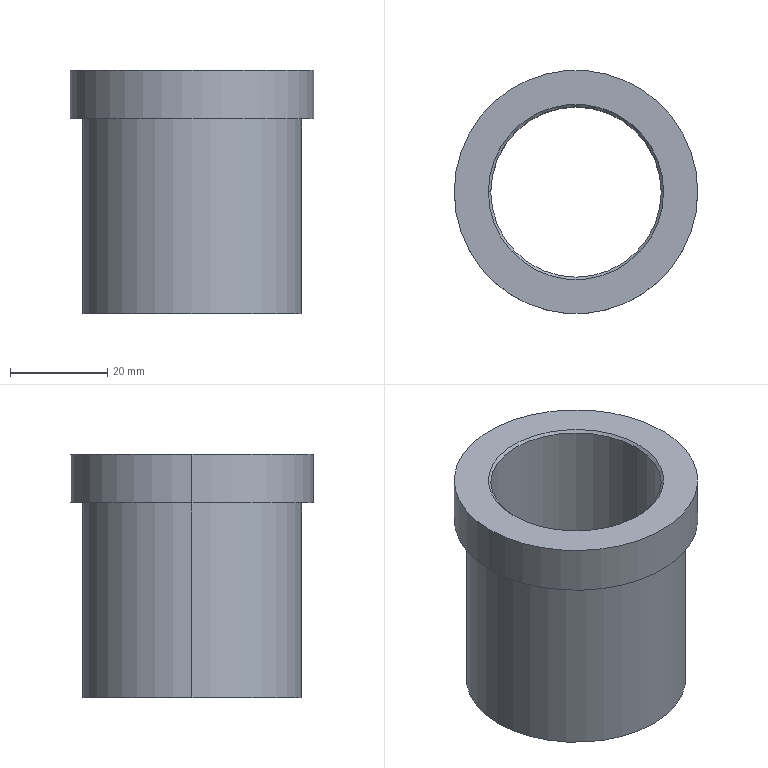Part | SolidWorks | features ICE 2, Chamfer 1, Extrusion 1 | 1 solid | 11 faces | box 50 x 50 x 50 mm | volume 35133 mm3 | cylinder 6 | plane 3 | cone 2 | commonest cylinder face diameters 35 x2 45 x2 50 x2
STEP:
#1=CARTESIAN_POINT('',(-17.5,0.,9.5));
#2=VERTEX_POINT('',#1);
#3=CARTESIAN_POINT('',(17.5,0.,9.5));
#4=VERTEX_POINT('',#3);
#5=CARTESIAN_POINT('',(0.,0.,9.5));
#6=DIRECTION('',(0.,0.,1.));
#7=DIRECTION('',(1.,0.,0.));
#8=AXIS2_PLACEMENT_3D('',#5,#6,#7);
#9=CIRCLE('',#8,17.5);
#10=EDGE_CURVE('',#2,#4,#9,.T.);
#11=ORIENTED_EDGE('',*,*,#10,.F.);
#12=CARTESIAN_POINT('',(-18.,0.,10.));
#13=VERTEX_POINT('',#12);
#14=CARTESIAN_POINT('',(-17.5,0.,9.5));
#15=DIRECTION('',(-0.7071,0.,0.7071));
#16=VECTOR('',#15,1000.);
#17=LINE('',#14,#16);
#18=EDGE_CURVE('',#2,#13,#17,.T.);
#19=ORIENTED_EDGE('',*,*,#18,.T.);
#20=CARTESIAN_POINT('',(18.,0.,10.));
#21=VERTEX_POINT('',#20);
#22=CARTESIAN_POINT('',(0.,0.,10.));
#23=DIRECTION('',(0.,0.,-1.));
#24=DIRECTION('',(1.,0.,0.));
#25=AXIS2_PLACEMENT_3D('',#22,#23,#24);
#26=CIRCLE('',#25,18.);
#27=EDGE_CURVE('',#21,#13,#26,.T.);
#28=ORIENTED_EDGE('',*,*,#27,.F.);
#29=CARTESIAN_POINT('',(17.5,0.,9.5));
#30=DIRECTION('',(0.7071,0.,0.7071));
#31=VECTOR('',#30,1000.);
#32=LINE('',#29,#31);
#33=EDGE_CURVE('',#4,#21,#32,.T.);
#34=ORIENTED_EDGE('',*,*,#33,.F.);
#35=EDGE_LOOP('',(#11,#19,#28,#34));
#36=FACE_OUTER_BOUND('',#35,.T.);
#37=CARTESIAN_POINT('',(0.,0.,9.5));
#38=DIRECTION('',(0.,0.,1.));
#39=DIRECTION('',(1.,0.,0.));
#40=AXIS2_PLACEMENT_3D('',#37,#38,#39);
#41=CONICAL_SURFACE('',#40,17.5,0.7854);
#42=ADVANCED_FACE('',(#36),#41,.F.);
#43=ORIENTED_EDGE('',*,*,#10,.T.);
#44=CARTESIAN_POINT('',(17.5,0.,-40.));
#45=VERTEX_POINT('',#44);
#46=CARTESIAN_POINT('',(17.5,0.,40.));
#47=DIRECTION('',(0.,0.,-1.));
#48=VECTOR('',#47,1000.);
#49=LINE('',#46,#48);
#50=EDGE_CURVE('',#4,#45,#49,.T.);
#51=ORIENTED_EDGE('',*,*,#50,.T.);
#52=CARTESIAN_POINT('',(-17.5,0.,-40.));
#53=VERTEX_POINT('',#52);
#54=CARTESIAN_POINT('',(0.,0.,-40.));
#55=DIRECTION('',(0.,0.,-1.));
#56=DIRECTION('',(-1.,0.,0.));
#57=AXIS2_PLACEMENT_3D('',#54,#55,#56);
#58=CIRCLE('',#57,17.5);
#59=EDGE_CURVE('',#45,#53,#58,.T.);
#60=ORIENTED_EDGE('',*,*,#59,.T.);
#61=CARTESIAN_POINT('',(-17.5,0.,40.));
#62=DIRECTION('',(0.,0.,-1.));
#63=VECTOR('',#62,1000.);
#64=LINE('',#61,#63);
#65=EDGE_CURVE('',#2,#53,#64,.T.);
#66=ORIENTED_EDGE('',*,*,#65,.F.);
#67=EDGE_LOOP('',(#43,#51,#60,#66));
#68=FACE_OUTER_BOUND('',#67,.T.);
#69=CARTESIAN_POINT('',(0.,0.,40.));
#70=DIRECTION('',(0.,0.,-1.));
#71=DIRECTION('',(-1.,0.,0.));
#72=AXIS2_PLACEMENT_3D('',#69,#70,#71);
#73=CYLINDRICAL_SURFACE('',#72,17.5);
#74=ADVANCED_FACE('',(#68),#73,.F.);
#75=CARTESIAN_POINT('',(-22.5,0.,-40.));
#76=VERTEX_POINT('',#75);
#77=CARTESIAN_POINT('',(22.5,0.,-40.));
#78=VERTEX_POINT('',#77);
#79=CARTESIAN_POINT('',(0.,0.,-40.));
#80=DIRECTION('',(0.,0.,-1.));
#81=DIRECTION('',(-1.,0.,0.));
#82=AXIS2_PLACEMENT_3D('',#79,#80,#81);
#83=CIRCLE('',#82,22.5);
#84=EDGE_CURVE('',#76,#78,#83,.T.);
#85=ORIENTED_EDGE('',*,*,#84,.F.);
#86=CARTESIAN_POINT('',(-22.5,0.,0.));
#87=VERTEX_POINT('',#86);
#88=CARTESIAN_POINT('',(-22.5,0.,-40.));
#89=DIRECTION('',(0.,0.,1.));
#90=VECTOR('',#89,1000.);
#91=LINE('',#88,#90);
#92=EDGE_CURVE('',#76,#87,#91,.T.);
#93=ORIENTED_EDGE('',*,*,#92,.T.);
#94=CARTESIAN_POINT('',(22.5,0.,0.));
#95=VERTEX_POINT('',#94);
#96=CARTESIAN_POINT('',(0.,0.,0.));
#97=DIRECTION('',(0.,0.,-1.));
#98=DIRECTION('',(-1.,0.,0.));
#99=AXIS2_PLACEMENT_3D('',#96,#97,#98);
#100=CIRCLE('',#99,22.5);
#101=EDGE_CURVE('',#87,#95,#100,.T.);
#102=ORIENTED_EDGE('',*,*,#101,.T.);
#103=CARTESIAN_POINT('',(22.5,0.,-40.));
#104=DIRECTION('',(0.,0.,1.));
#105=VECTOR('',#104,1000.);
#106=LINE('',#103,#105);
#107=EDGE_CURVE('',#78,#95,#106,.T.);
#108=ORIENTED_EDGE('',*,*,#107,.F.);
#109=EDGE_LOOP('',(#85,#93,#102,#108));
#110=FACE_OUTER_BOUND('',#109,.T.);
#111=CARTESIAN_POINT('',(0.,0.,-40.));
#112=DIRECTION('',(0.,0.,1.));
#113=DIRECTION('',(1.,0.,0.));
#114=AXIS2_PLACEMENT_3D('',#111,#112,#113);
#115=CYLINDRICAL_SURFACE('',#114,22.5);
#116=ADVANCED_FACE('',(#110),#115,.T.);
#117=CARTESIAN_POINT('',(25.,0.,10.));
#118=VERTEX_POINT('',#117);
#119=CARTESIAN_POINT('',(-25.,0.,10.));
#120=VERTEX_POINT('',#119);
#121=CARTESIAN_POINT('',(0.,0.,10.));
#122=DIRECTION('',(0.,0.,1.));
#123=DIRECTION('',(1.,0.,0.));
#124=AXIS2_PLACEMENT_3D('',#121,#122,#123);
#125=CIRCLE('',#124,25.);
#126=EDGE_CURVE('',#118,#120,#125,.T.);
#127=ORIENTED_EDGE('',*,*,#126,.F.);
#128=CARTESIAN_POINT('',(25.,0.,0.));
#129=VERTEX_POINT('',#128);
#130=CARTESIAN_POINT('',(25.,0.,10.));
#131=DIRECTION('',(0.,0.,-1.));
#132=VECTOR('',#131,1000.);
#133=LINE('',#130,#132);
#134=EDGE_CURVE('',#118,#129,#133,.T.);
#135=ORIENTED_EDGE('',*,*,#134,.T.);
#136=CARTESIAN_POINT('',(-25.,0.,0.));
#137=VERTEX_POINT('',#136);
#138=CARTESIAN_POINT('',(0.,0.,0.));
#139=DIRECTION('',(0.,0.,1.));
#140=DIRECTION('',(1.,0.,0.));
#141=AXIS2_PLACEMENT_3D('',#138,#139,#140);
#142=CIRCLE('',#141,25.);
#143=EDGE_CURVE('',#129,#137,#142,.T.);
#144=ORIENTED_EDGE('',*,*,#143,.T.);
#145=CARTESIAN_POINT('',(-25.,0.,10.));
#146=DIRECTION('',(0.,0.,-1.));
#147=VECTOR('',#146,1000.);
#148=LINE('',#145,#147);
#149=EDGE_CURVE('',#120,#137,#148,.T.);
#150=ORIENTED_EDGE('',*,*,#149,.F.);
#151=EDGE_LOOP('',(#127,#135,#144,#150));
#152=FACE_OUTER_BOUND('',#151,.T.);
#153=CARTESIAN_POINT('',(0.,0.,10.));
#154=DIRECTION('',(0.,0.,-1.));
#155=DIRECTION('',(-1.,0.,0.));
#156=AXIS2_PLACEMENT_3D('',#153,#154,#155);
#157=CYLINDRICAL_SURFACE('',#156,25.);
#158=ADVANCED_FACE('',(#152),#157,.T.);
#159=ORIENTED_EDGE('',*,*,#134,.F.);
#160=CARTESIAN_POINT('',(0.,0.,10.));
#161=DIRECTION('',(0.,0.,1.));
#162=DIRECTION('',(1.,0.,0.));
#163=AXIS2_PLACEMENT_3D('',#160,#161,#162);
#164=CIRCLE('',#163,25.);
#165=EDGE_CURVE('',#120,#118,#164,.T.);
#166=ORIENTED_EDGE('',*,*,#165,.F.);
#167=ORIENTED_EDGE('',*,*,#149,.T.);
#168=CARTESIAN_POINT('',(0.,0.,0.));
#169=DIRECTION('',(0.,0.,1.));
#170=DIRECTION('',(1.,0.,0.));
#171=AXIS2_PLACEMENT_3D('',#168,#169,#170);
#172=CIRCLE('',#171,25.);
#173=EDGE_CURVE('',#137,#129,#172,.T.);
#174=ORIENTED_EDGE('',*,*,#173,.T.);
#175=EDGE_LOOP('',(#159,#166,#167,#174));
#176=FACE_OUTER_BOUND('',#175,.T.);
#177=CARTESIAN_POINT('',(0.,0.,10.));
#178=DIRECTION('',(0.,0.,-1.));
#179=DIRECTION('',(-1.,0.,0.));
#180=AXIS2_PLACEMENT_3D('',#177,#178,#179);
#181=CYLINDRICAL_SURFACE('',#180,25.);
#182=ADVANCED_FACE('',(#176),#181,.T.);
#183=ORIENTED_EDGE('',*,*,#27,.T.);
#184=CARTESIAN_POINT('',(0.,0.,10.));
#185=DIRECTION('',(0.,0.,-1.));
#186=DIRECTION('',(1.,0.,0.));
#187=AXIS2_PLACEMENT_3D('',#184,#185,#186);
#188=CIRCLE('',#187,18.);
#189=EDGE_CURVE('',#13,#21,#188,.T.);
#190=ORIENTED_EDGE('',*,*,#189,.T.);
#191=EDGE_LOOP('',(#183,#190));
#192=FACE_BOUND('',#191,.T.);
#193=ORIENTED_EDGE('',*,*,#165,.T.);
#194=ORIENTED_EDGE('',*,*,#126,.T.);
#195=EDGE_LOOP('',(#193,#194));
#196=FACE_OUTER_BOUND('',#195,.T.);
#197=CARTESIAN_POINT('',(0.,0.,10.));
#198=DIRECTION('',(0.,0.,1.));
#199=DIRECTION('',(1.,0.,0.));
#200=AXIS2_PLACEMENT_3D('',#197,#198,#199);
#201=PLANE('',#200);
#202=ADVANCED_FACE('',(#192,#196),#201,.T.);
#203=CARTESIAN_POINT('',(0.,0.,0.));
#204=DIRECTION('',(0.,0.,-1.));
#205=DIRECTION('',(-1.,0.,0.));
#206=AXIS2_PLACEMENT_3D('',#203,#204,#205);
#207=CIRCLE('',#206,22.5);
#208=EDGE_CURVE('',#95,#87,#207,.T.);
#209=ORIENTED_EDGE('',*,*,#208,.F.);
#210=ORIENTED_EDGE('',*,*,#101,.F.);
#211=EDGE_LOOP('',(#209,#210));
#212=FACE_BOUND('',#211,.T.);
#213=ORIENTED_EDGE('',*,*,#173,.F.);
#214=ORIENTED_EDGE('',*,*,#143,.F.);
#215=EDGE_LOOP('',(#213,#214));
#216=FACE_OUTER_BOUND('',#215,.T.);
#217=CARTESIAN_POINT('',(0.,0.,0.));
#218=DIRECTION('',(0.,0.,1.));
#219=DIRECTION('',(1.,0.,0.));
#220=AXIS2_PLACEMENT_3D('',#217,#218,#219);
#221=PLANE('',#220);
#222=ADVANCED_FACE('',(#212,#216),#221,.F.);
#223=ORIENTED_EDGE('',*,*,#92,.F.);
#224=CARTESIAN_POINT('',(0.,0.,-40.));
#225=DIRECTION('',(0.,0.,-1.));
#226=DIRECTION('',(-1.,0.,0.));
#227=AXIS2_PLACEMENT_3D('',#224,#225,#226);
#228=CIRCLE('',#227,22.5);
#229=EDGE_CURVE('',#78,#76,#228,.T.);
#230=ORIENTED_EDGE('',*,*,#229,.F.);
#231=ORIENTED_EDGE('',*,*,#107,.T.);
#232=ORIENTED_EDGE('',*,*,#208,.T.);
#233=EDGE_LOOP('',(#223,#230,#231,#232));
#234=FACE_OUTER_BOUND('',#233,.T.);
#235=CARTESIAN_POINT('',(0.,0.,-40.));
#236=DIRECTION('',(0.,0.,1.));
#237=DIRECTION('',(1.,0.,0.));
#238=AXIS2_PLACEMENT_3D('',#235,#236,#237);
#239=CYLINDRICAL_SURFACE('',#238,22.5);
#240=ADVANCED_FACE('',(#234),#239,.T.);
#241=CARTESIAN_POINT('',(0.,0.,-40.));
#242=DIRECTION('',(0.,0.,-1.));
#243=DIRECTION('',(-1.,0.,0.));
#244=AXIS2_PLACEMENT_3D('',#241,#242,#243);
#245=CIRCLE('',#244,17.5);
#246=EDGE_CURVE('',#53,#45,#245,.T.);
#247=ORIENTED_EDGE('',*,*,#246,.F.);
#248=ORIENTED_EDGE('',*,*,#59,.F.);
#249=EDGE_LOOP('',(#247,#248));
#250=FACE_BOUND('',#249,.T.);
#251=ORIENTED_EDGE('',*,*,#229,.T.);
#252=ORIENTED_EDGE('',*,*,#84,.T.);
#253=EDGE_LOOP('',(#251,#252));
#254=FACE_OUTER_BOUND('',#253,.T.);
#255=CARTESIAN_POINT('',(0.,0.,-40.));
#256=DIRECTION('',(0.,0.,-1.));
#257=DIRECTION('',(-1.,0.,0.));
#258=AXIS2_PLACEMENT_3D('',#255,#256,#257);
#259=PLANE('',#258);
#260=ADVANCED_FACE('',(#250,#254),#259,.T.);
#261=ORIENTED_EDGE('',*,*,#50,.F.);
#262=CARTESIAN_POINT('',(0.,0.,9.5));
#263=DIRECTION('',(0.,0.,1.));
#264=DIRECTION('',(1.,0.,0.));
#265=AXIS2_PLACEMENT_3D('',#262,#263,#264);
#266=CIRCLE('',#265,17.5);
#267=EDGE_CURVE('',#4,#2,#266,.T.);
#268=ORIENTED_EDGE('',*,*,#267,.T.);
#269=ORIENTED_EDGE('',*,*,#65,.T.);
#270=ORIENTED_EDGE('',*,*,#246,.T.);
#271=EDGE_LOOP('',(#261,#268,#269,#270));
#272=FACE_OUTER_BOUND('',#271,.T.);
#273=CARTESIAN_POINT('',(0.,0.,40.));
#274=DIRECTION('',(0.,0.,-1.));
#275=DIRECTION('',(-1.,0.,0.));
#276=AXIS2_PLACEMENT_3D('',#273,#274,#275);
#277=CYLINDRICAL_SURFACE('',#276,17.5);
#278=ADVANCED_FACE('',(#272),#277,.F.);
#279=ORIENTED_EDGE('',*,*,#18,.F.);
#280=ORIENTED_EDGE('',*,*,#267,.F.);
#281=ORIENTED_EDGE('',*,*,#33,.T.);
#282=ORIENTED_EDGE('',*,*,#189,.F.);
#283=EDGE_LOOP('',(#279,#280,#281,#282));
#284=FACE_OUTER_BOUND('',#283,.T.);
#285=CARTESIAN_POINT('',(0.,0.,9.5));
#286=DIRECTION('',(0.,0.,1.));
#287=DIRECTION('',(1.,0.,0.));
#288=AXIS2_PLACEMENT_3D('',#285,#286,#287);
#289=CONICAL_SURFACE('',#288,17.5,0.7854);
#290=ADVANCED_FACE('',(#284),#289,.F.);
#291=CLOSED_SHELL('',(#42,#74,#116,#158,#182,#202,#222,#240,#260,#278,#290));
#292=MANIFOLD_SOLID_BREP('',#291);
#293=CARTESIAN_POINT('',(0.,0.,0.));
#294=DIRECTION('',(0.,0.,1.));
#295=DIRECTION('',(1.,0.,0.));
#296=AXIS2_PLACEMENT_3D('',#293,#294,#295);
#297=(LENGTH_UNIT()NAMED_UNIT(*)SI_UNIT(.MILLI.,.METRE.));
#298=UNCERTAINTY_MEASURE_WITH_UNIT(LENGTH_MEASURE(0.00001),#297,'','');
#299=(NAMED_UNIT(*)PLANE_ANGLE_UNIT()SI_UNIT($,.RADIAN.));
#300=(NAMED_UNIT(*)SI_UNIT($,.STERADIAN.)SOLID_ANGLE_UNIT());
#301=(GEOMETRIC_REPRESENTATION_CONTEXT(3)GLOBAL_UNCERTAINTY_ASSIGNED_CONTEXT((#298))GLOBAL_UNIT_ASSIGNED_CONTEXT((#297,#299,#300))REPRESENTATION_CONTEXT('',''));
#302=ADVANCED_BREP_SHAPE_REPRESENTATION('',(#292,#296),#301);